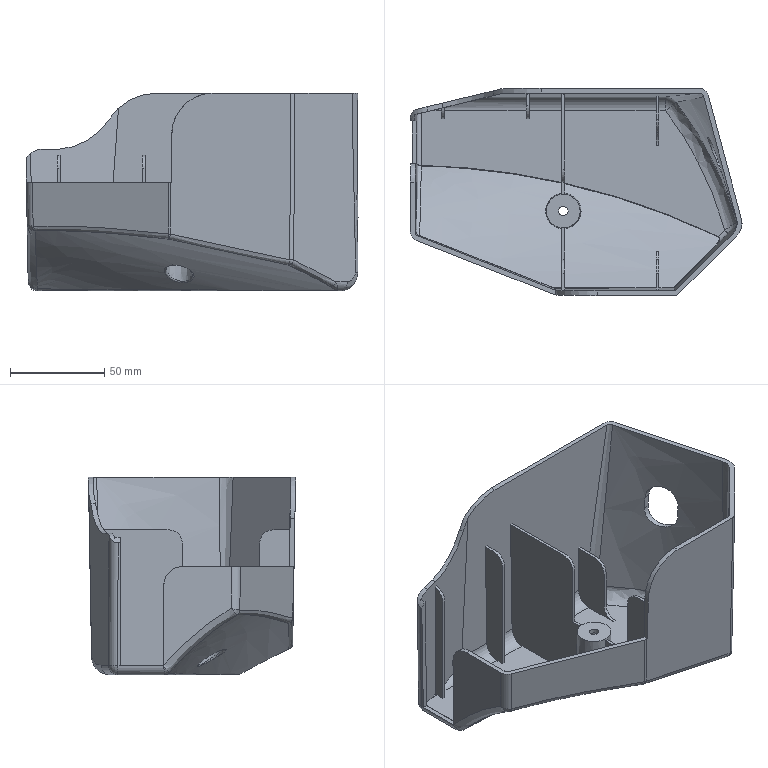Part | STEP file | HHJR | 1 solid | 136 faces | box 176.285 x 110 x 105.001 mm | volume 141241 mm3 | plane 54 | spline 43 | cylinder 32 | sphere 5 | cone 2 | commonest cylinder face diameters 10 x6 14 x6 15 x5 5 x4 20 x3 1 x2